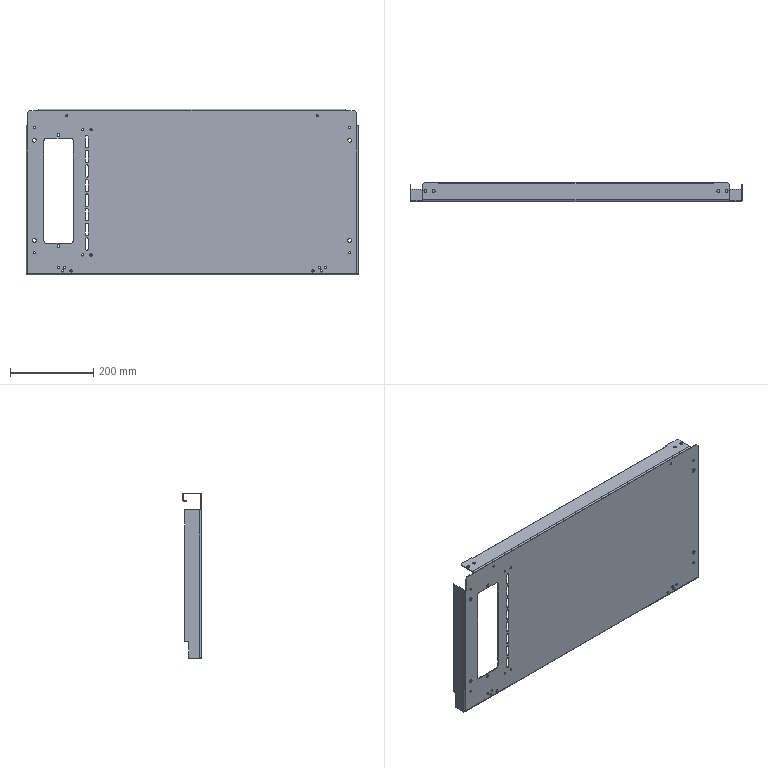Part | STEP file | 1 solid | 188 faces | box 796 x 45 x 398 mm | volume 779012 mm3 | cylinder 102 | plane 86 | commonest cylinder face diameters 5.3 x42 7 x42 9 x8 3 x6 13 x4